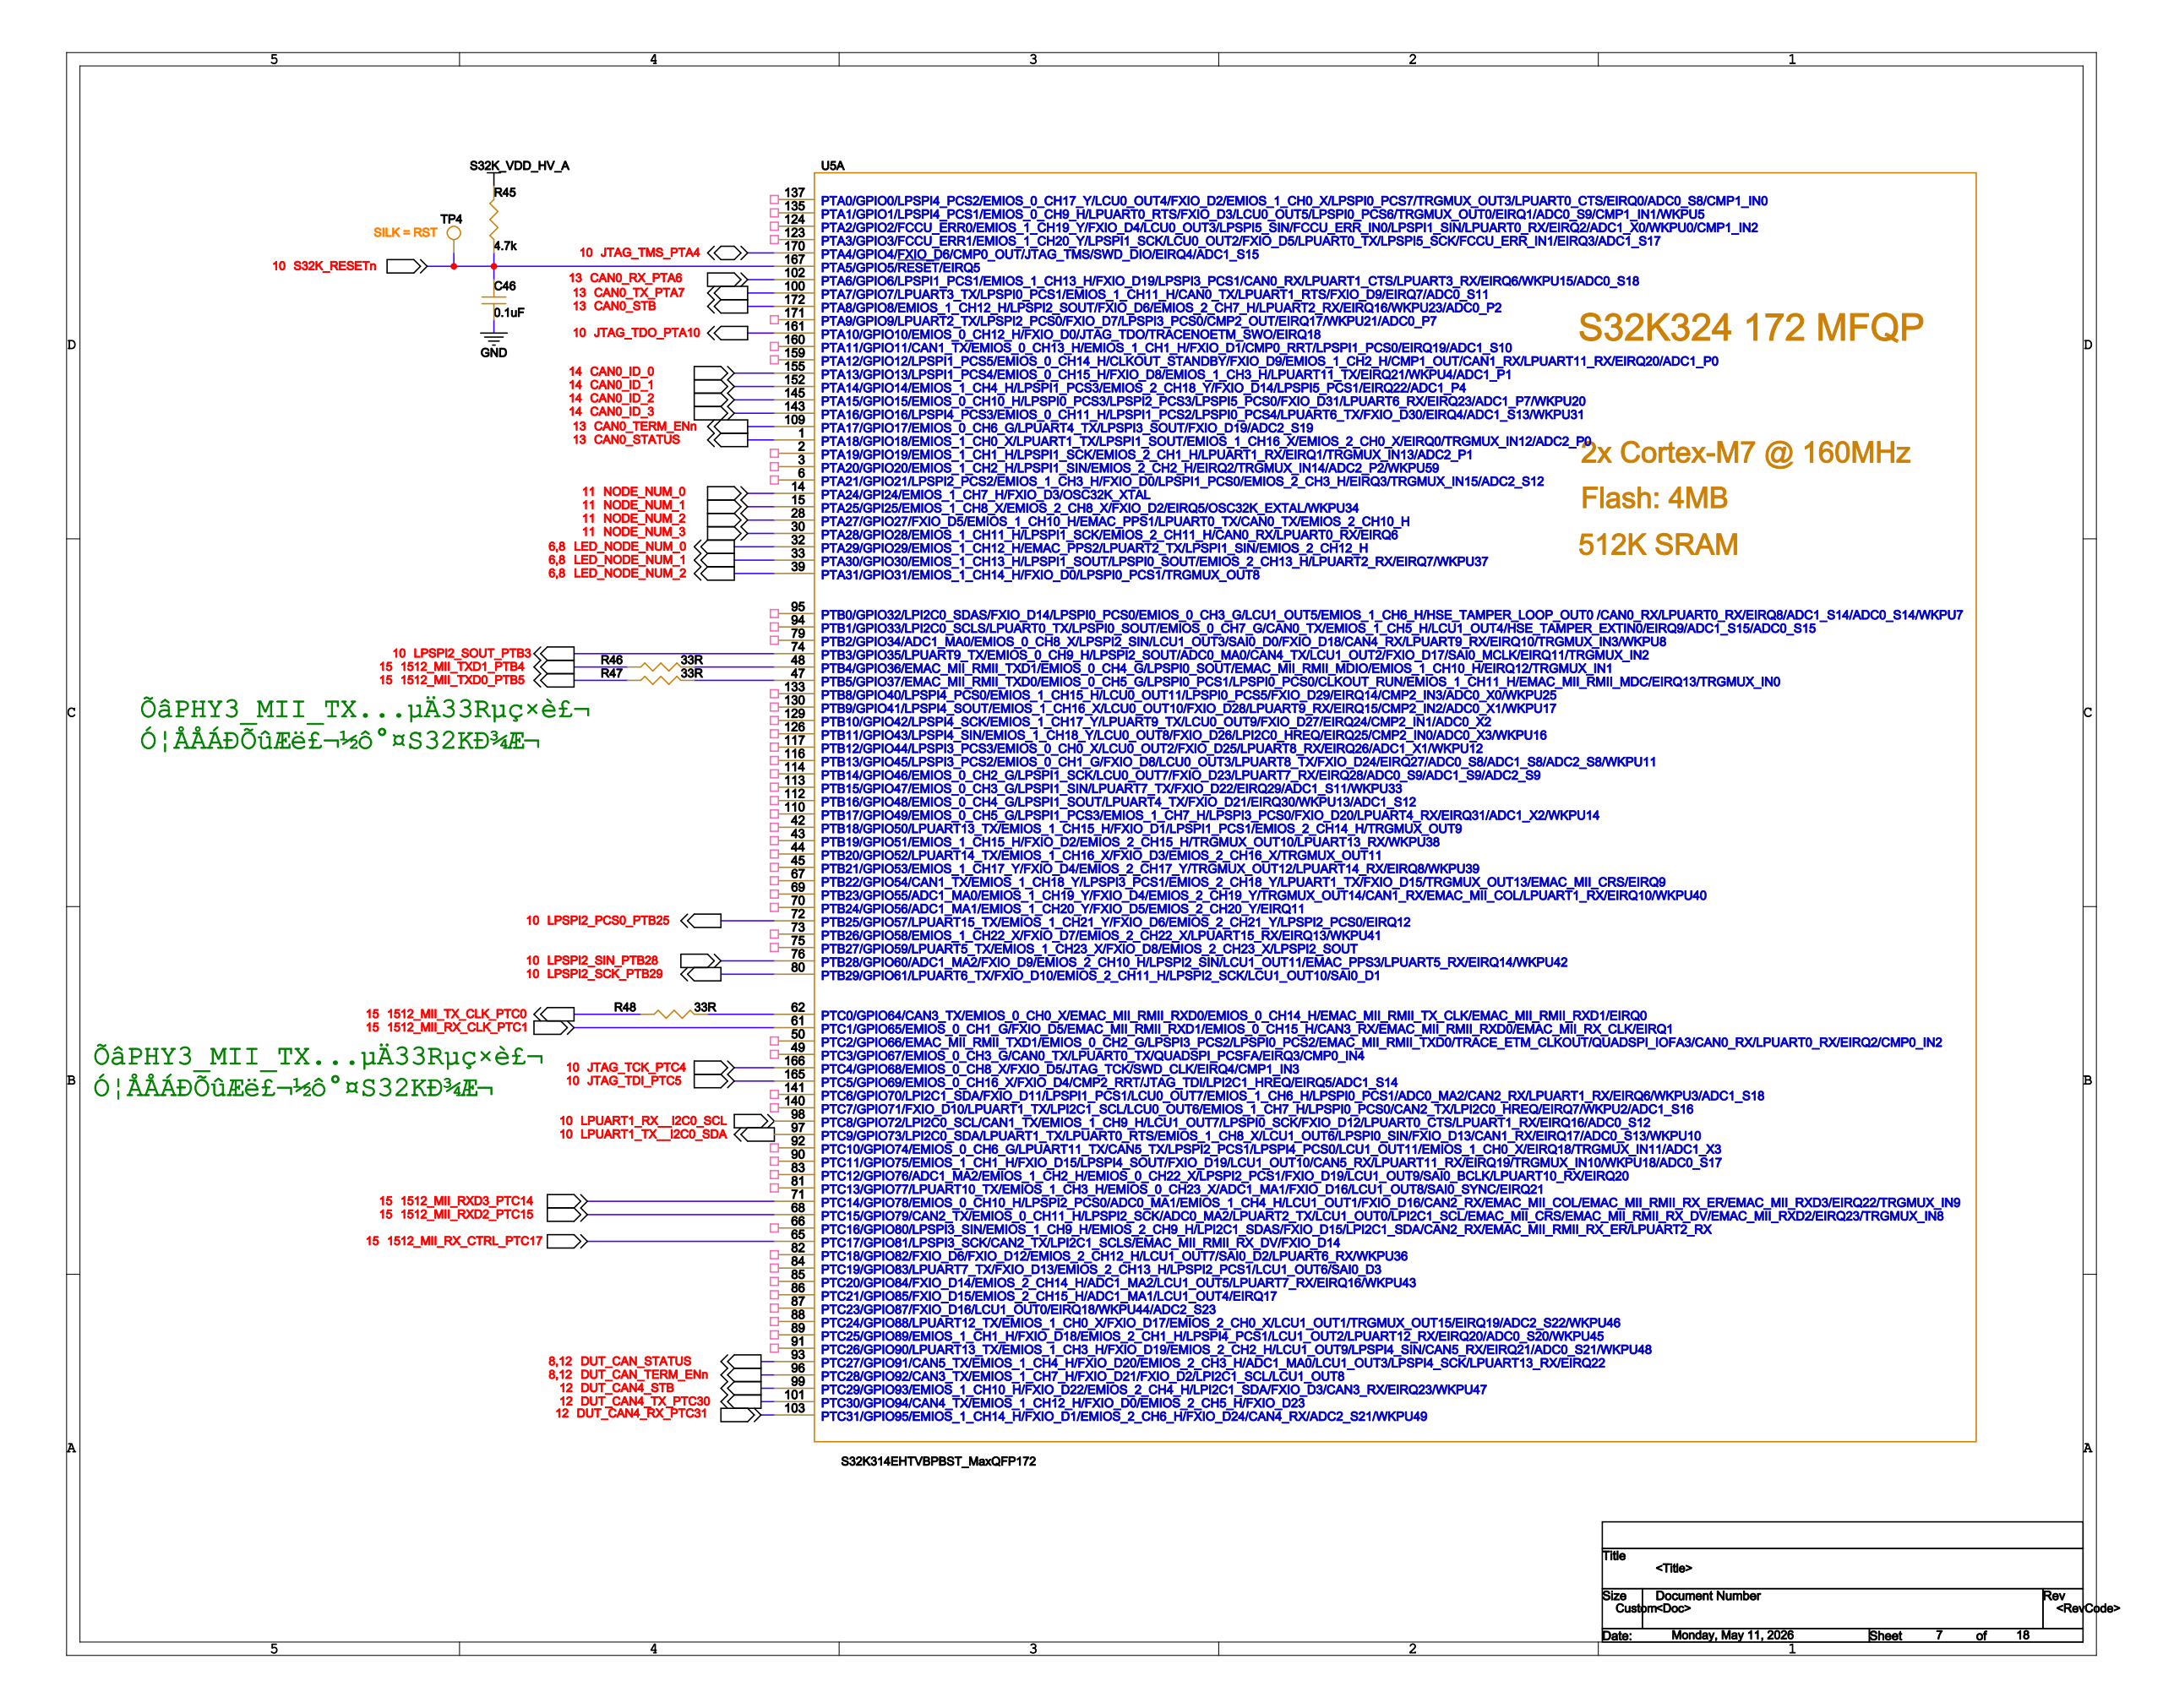Circuit board | Cadence Allegro | 330 parts | 215 nets | one sheet of the schematic
Parts on this sheet (reference | value | footprint):
C46 | 0.1uF | 0402
R45 | 4.7K | 0402
R46 | 33R | 0402
R47 | 33R | 0402
R48 | 33R | 0402
TP4 | TP | S0400CI
U5 | S32K314EHTVBPBST_MaxQFP172 | MQFP172_0P65_16X16
Nets of these parts (net: part-pin ...):
GND: C46-1
DUT_CAN4_STB: U5-99
CAN0_STB: U5-172
S32K_VDD_HV_A: R45-1 U5-18
S32K_RESETN: C46-2 R45-2 TP4-1 U5-167
LPUART1_TX__I2C0_SDA: U5-97
LPUART1_RX__I2C0_SCL: U5-98
CAN0_ID_0: U5-155
JTAG_TCK_PTC4: U5-166
JTAG_TDO_PTA10: U5-161
JTAG_TMS_PTA4: U5-170
JTAG_TDI_PTC5: U5-165
LPSPI2_PCS0_PTB25: U5-72
NODE_NUM_1: U5-15
NODE_NUM_0: U5-14
NODE_NUM_2: U5-28
NODE_NUM_3: U5-30
CAN0_ID_3: U5-143
CAN0_ID_2: U5-145
CAN0_ID_1: U5-152
1512_MII_RX_CLK_PTC1: U5-61
1512_MII_RXD2_PTC15: U5-68
1512_MII_RXD3_PTC14: U5-71
1512_MII_RX_CTRL_PTC17: U5-65
1512_MII_TXD1_PTB4: R46-1
N2514309: R46-2 U5-48
1512_MII_TXD0_PTB5: R47-1
N2514313: R47-2 U5-47
1512_MII_TX_CLK_PTC0: R48-1
N2514360: R48-2 U5-62
DUT_CAN4_RX_PTC31: U5-103
DUT_CAN4_TX_PTC30: U5-101
CAN0_RX_PTA6: U5-102
CAN0_TX_PTA7: U5-100
CAN0_STATUS: U5-1
LED_NODE_NUM_0: U5-32
LED_NODE_NUM_1: U5-33
LED_NODE_NUM_2: U5-39
LPSPI2_SIN_PTB28: U5-76
LPSPI2_SCK_PTB29: U5-80
LPSPI2_SOUT_PTB3: U5-74
DUT_CAN_STATUS: U5-93